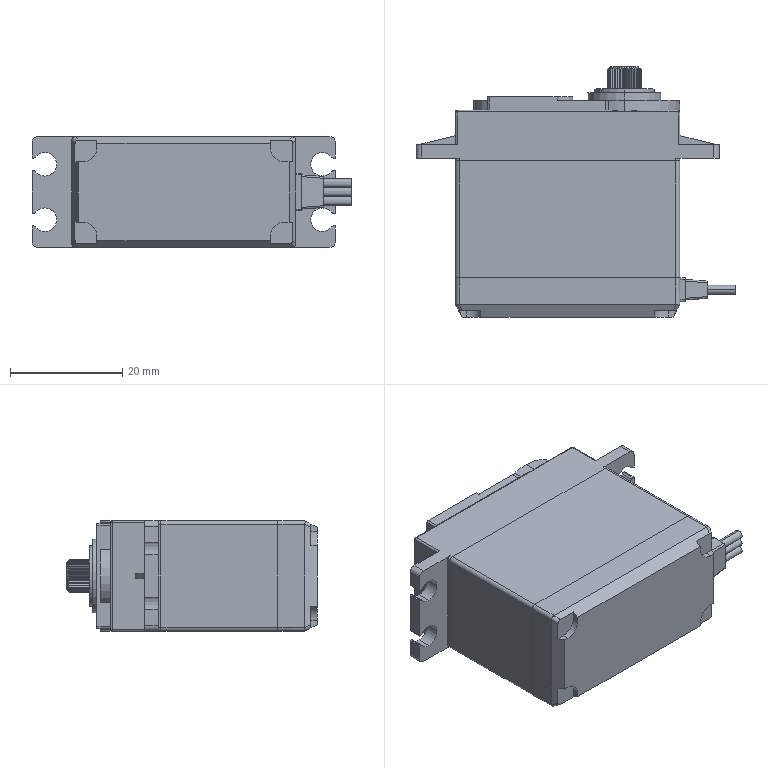Part | SolidWorks | features BaseBody 8 | 8 solids | 373 faces | box 56.95 x 44.55 x 19.7 mm | volume 5255 mm3 | plane 225 | cylinder 142 | spline 4 | cone 2 | commonest cylinder face diameters 0.6 x39 5.95 x36 1.4 x16 4.2 x12 1 x8 1.6 x6